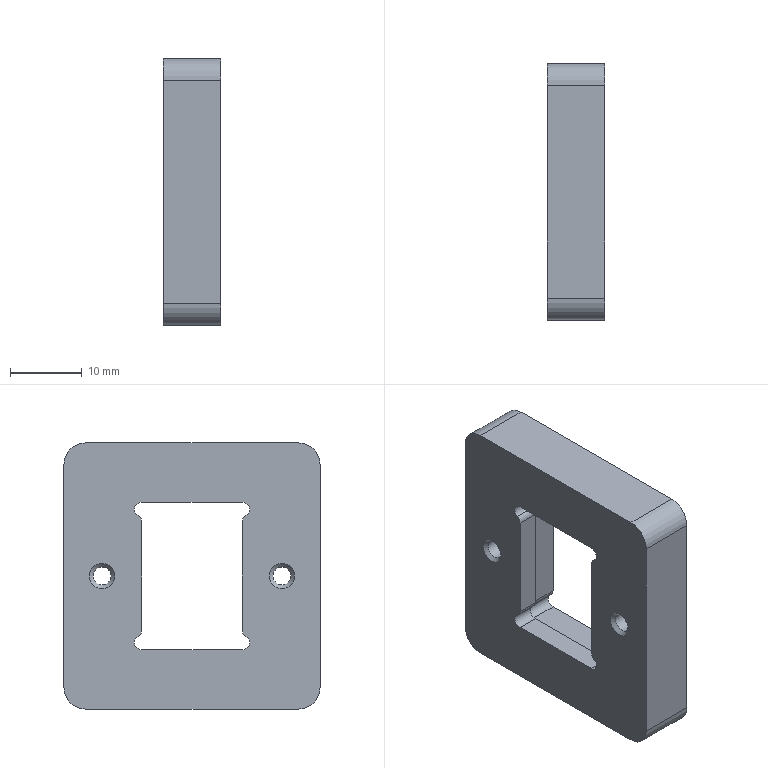CAM job | NX | 3+2 milling, drilling | part box 8 x 35.6 x 37 mm | stock box 10 x 40.6 x 42 mm
Tools:
number,name,description,diameter,corner_radius,flute_length,length,flutes
9,D10,平底铣刀-粗,10.0,0.0,35.0,75.0,2
11,D2-J,平底铣刀-精,2.0,0.0,50.0,75.0,2
7,D6-J,平底铣刀-精,6.0,0.0,25.0,75.0,2
10,D10-J,平底铣刀-精,10.0,0.0,35.0,75.0,2
1,D80R0.8飞刀,圆鼻刀-粗,80.0,0.8,50.0,75.0,2
2,D6倒角刀,倒角刀,6.0,0.0,3.0,25.0,2
20,M3X0.5,丝锥,2.5,0.0,35.0,50.0,2
12,ZT2.5,钻头,2.5,0.0,35.0,50.0,2
Operations:
program,operation,operation_type,tool,method,geometry_group,spindle_rpm,surface_speed,feed_per_tooth,feed_cut,feed_plunge,cut_length_mm,path_length_mm,cut_time_min,machine_time_min
B,面铣自动飞面开粗一刀_COPY,FaceMilling,D80R0.8飞刀,分层开粗-切深K-步距G,W-B,4500.0,890.615,0.3333,3000.0,100.0,725.0,1336.64,0.2417,0.3028
B,面铣自动飞面精光一刀_COPY,FaceMilling,D80R0.8飞刀,侧刃精光-切深K-步距G,W-B,4500.0,890.615,0.1111,1000.0,100.0,145.0,181.0,0.145,0.1486
B,钻倒角_2,Operation,D6倒角刀,METHOD,W-B,8000.0,150.796,0.0625,1000.0,0.0,9.5,87.179,0.0095,0.0173
B,平面去毛刺6X45L_COPY,SurfaceContour,D6倒角刀,爬面_倒角-切深0-步距G,W-B,6500.0,122.519,0.1154,1500.0,100.0,220.082,300.642,0.1467,0.1548
A,顶面,FaceMilling,D80R0.8飞刀,侧刃精光-切深K-步距G,W-A,4000.0,1005.31,0.125,1000.0,100.0,131.0,167.0,0.131,0.1346
A,外形粗_2,VolumeBased25DMillingOperation,D10,METHOD,W-A,8000.0,251.327,0.3125,5000.0,80.0,2066.645,2113.245,0.4133,0.418
A,底壁铣螺旋开粗-中_COPY,VolumeBased25DMillingOperation,D10,分层开粗-切深K-步距G,W-A,8000.0,251.327,0.125,2000.0,100.0,647.728,690.628,0.3239,0.3282
A,腰槽粗_1,VolumeBased25DMillingOperation,D10,METHOD,W-A,6000.0,113.0,0.2083,2500.0,100.0,424.52,476.52,0.1698,0.175
A,打点-深0.8,Operation,D6倒角刀,NONE,W-A,8000.0,150.796,0.0312,500.0,90.0,3.6,73.22,0.0072,0.0142
A,通孔-M3螺纹底孔,Operation,ZT2.5,NONE,W-A,3000.0,23.562,0.05,300.0,90.0,29.502,125.024,0.0983,0.1079
A,清角D4,ZLevelMilling,D2-J,METHOD,W-A,8000.0,50.266,0.125,2000.0,80.0,1534.555,1635.301,0.768,0.7781
A,清角D4_2,ZLevelMilling,D2-J,METHOD,W-A,8000.0,50.266,0.125,2000.0,80.0,917.906,1002.665,0.4595,0.468
A,仅选体,SurfaceContour,D6倒角刀,METHOD,W-A,8000.0,150.796,0.1875,3000.0,100.0,238.559,332.065,0.0795,0.0889
A,钻倒角_1,Operation,D6倒角刀,METHOD,W-A,8000.0,150.796,0.0312,500.0,0.0,9.5,87.179,0.019,0.0268
A,通孔-攻牙M3,Operation,M3X0.5,METHOD,W-A,800.0,6.283,0.0003,0.5,90.0,23.0,113.02,46.0,46.009
A,腰槽精_1,VolumeBased25DMillingOperation,D6-J,METHOD,W-A,6000.0,113.0,0.0667,600.0,100.0,47.228,102.628,0.0787,0.0843
A,底侧精_3,VolumeBased25DMillingOperation,D6-J,METHOD,W-A,6000.0,113.0,0.2083,1200.0,100.0,60.842,109.832,0.0507,0.0556
A,外形半精_2,VolumeBased25DMillingOperation,D10-J,METHOD,W-A,8000.0,251.327,0.0625,1000.0,100.0,176.452,231.851,0.1765,0.182